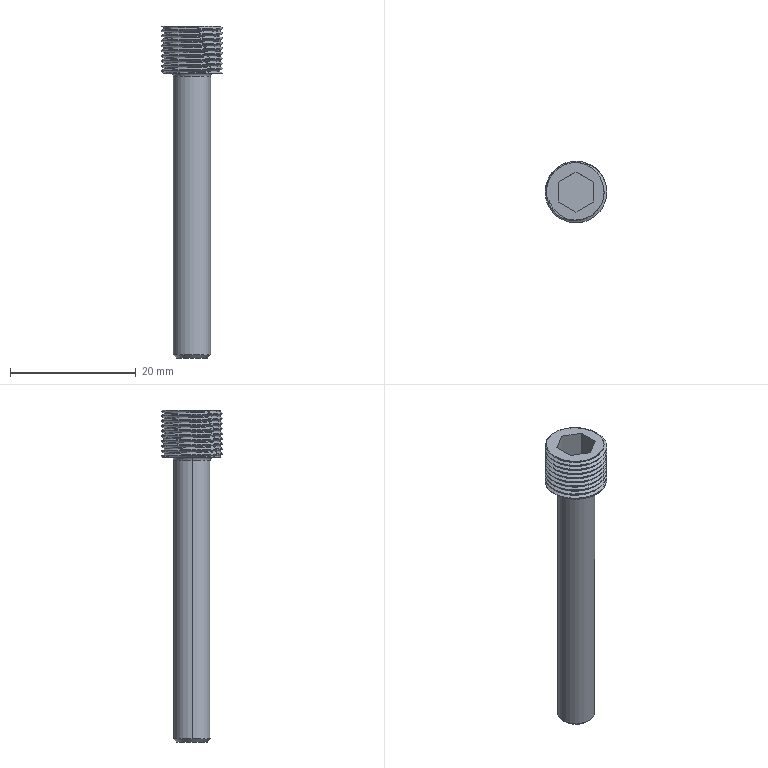Part | SolidWorks | features BaseBody 1 | 1 solid | 40 faces | box 9.8 x 9.8 x 52.75 mm | volume 1605 mm3 | cylinder 21 | plane 10 | cone 4 | spline 3 | torus 2 | commonest cylinder face diameters 9.8 x19 5.9 x2